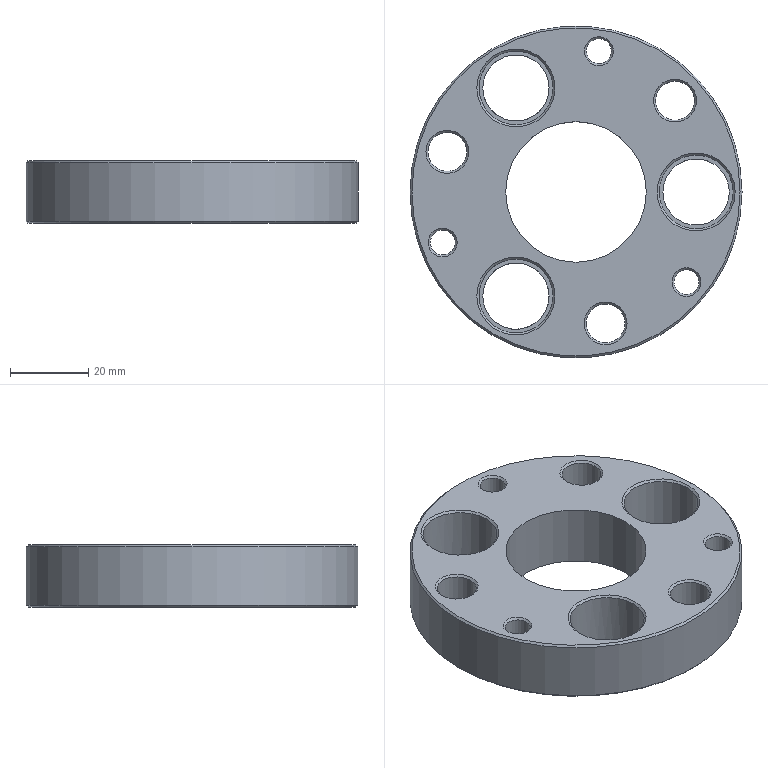Part | NX | features BREP 1 | 1 solid | 39 faces | box 85 x 85 x 16 mm | volume 54576 mm3 | cylinder 17 | cone 14 | plane 8 | commonest cylinder face diameters 6.4 x3 10 x3 10.5 x3 17 x3 19 x3 36 x1
STEP:
#1=CARTESIAN_POINT('',(-5.38,-26.639,16.));
#2=VERTEX_POINT('',#1);
#3=CARTESIAN_POINT('',(-15.38,-26.639,16.));
#4=DIRECTION('',(0.,0.,-1.));
#5=DIRECTION('',(1.,0.,0.));
#6=AXIS2_PLACEMENT_3D('',#3,#4,#5);
#7=CIRCLE('',#6,10.);
#8=EDGE_CURVE('',#2,#2,#7,.T.);
#9=ORIENTED_EDGE('',*,*,#8,.F.);
#10=EDGE_LOOP('',(#9));
#11=FACE_BOUND('',#10,.T.);
#12=CARTESIAN_POINT('',(-5.88,-26.639,15.5));
#13=VERTEX_POINT('',#12);
#14=CARTESIAN_POINT('',(-15.38,-26.639,15.5));
#15=DIRECTION('',(0.,0.,1.));
#16=DIRECTION('',(1.,0.,0.));
#17=AXIS2_PLACEMENT_3D('',#14,#15,#16);
#18=CIRCLE('',#17,9.5);
#19=EDGE_CURVE('',#13,#13,#18,.T.);
#20=ORIENTED_EDGE('',*,*,#19,.F.);
#21=EDGE_LOOP('',(#20));
#22=FACE_BOUND('',#21,.T.);
#23=CARTESIAN_POINT('',(-15.38,-26.639,16.));
#24=DIRECTION('',(0.,0.,1.));
#25=DIRECTION('',(1.,0.,0.));
#26=AXIS2_PLACEMENT_3D('',#23,#24,#25);
#27=CONICAL_SURFACE('',#26,10.,0.7854);
#28=ADVANCED_FACE('',(#11,#22),#27,.F.);
#29=CARTESIAN_POINT('',(-5.38,26.639,16.));
#30=VERTEX_POINT('',#29);
#31=CARTESIAN_POINT('',(-15.38,26.639,16.));
#32=DIRECTION('',(0.,0.,-1.));
#33=DIRECTION('',(1.,0.,0.));
#34=AXIS2_PLACEMENT_3D('',#31,#32,#33);
#35=CIRCLE('',#34,10.);
#36=EDGE_CURVE('',#30,#30,#35,.T.);
#37=ORIENTED_EDGE('',*,*,#36,.F.);
#38=EDGE_LOOP('',(#37));
#39=FACE_BOUND('',#38,.T.);
#40=CARTESIAN_POINT('',(-5.88,26.639,15.5));
#41=VERTEX_POINT('',#40);
#42=CARTESIAN_POINT('',(-15.38,26.639,15.5));
#43=DIRECTION('',(0.,0.,1.));
#44=DIRECTION('',(1.,0.,0.));
#45=AXIS2_PLACEMENT_3D('',#42,#43,#44);
#46=CIRCLE('',#45,9.5);
#47=EDGE_CURVE('',#41,#41,#46,.T.);
#48=ORIENTED_EDGE('',*,*,#47,.F.);
#49=EDGE_LOOP('',(#48));
#50=FACE_BOUND('',#49,.T.);
#51=CARTESIAN_POINT('',(-15.38,26.639,16.));
#52=DIRECTION('',(0.,0.,1.));
#53=DIRECTION('',(1.,0.,0.));
#54=AXIS2_PLACEMENT_3D('',#51,#52,#53);
#55=CONICAL_SURFACE('',#54,10.,0.7854);
#56=ADVANCED_FACE('',(#39,#50),#55,.F.);
#57=CARTESIAN_POINT('',(40.76,0.,16.));
#58=VERTEX_POINT('',#57);
#59=CARTESIAN_POINT('',(30.76,0.,16.));
#60=DIRECTION('',(0.,0.,-1.));
#61=DIRECTION('',(1.,0.,0.));
#62=AXIS2_PLACEMENT_3D('',#59,#60,#61);
#63=CIRCLE('',#62,10.);
#64=EDGE_CURVE('',#58,#58,#63,.T.);
#65=ORIENTED_EDGE('',*,*,#64,.F.);
#66=EDGE_LOOP('',(#65));
#67=FACE_BOUND('',#66,.T.);
#68=CARTESIAN_POINT('',(40.26,0.,15.5));
#69=VERTEX_POINT('',#68);
#70=CARTESIAN_POINT('',(30.76,0.,15.5));
#71=DIRECTION('',(0.,0.,1.));
#72=DIRECTION('',(1.,0.,0.));
#73=AXIS2_PLACEMENT_3D('',#70,#71,#72);
#74=CIRCLE('',#73,9.5);
#75=EDGE_CURVE('',#69,#69,#74,.T.);
#76=ORIENTED_EDGE('',*,*,#75,.F.);
#77=EDGE_LOOP('',(#76));
#78=FACE_BOUND('',#77,.T.);
#79=CARTESIAN_POINT('',(30.76,0.,16.));
#80=DIRECTION('',(0.,0.,1.));
#81=DIRECTION('',(1.,0.,0.));
#82=AXIS2_PLACEMENT_3D('',#79,#80,#81);
#83=CONICAL_SURFACE('',#82,10.,0.7854);
#84=ADVANCED_FACE('',(#67,#78),#83,.F.);
#85=CARTESIAN_POINT('',(0.5951,36.029,0.));
#86=VERTEX_POINT('',#85);
#87=CARTESIAN_POINT('',(5.845,36.029,0.));
#88=DIRECTION('',(0.,0.,-1.));
#89=DIRECTION('',(-1.,0.,0.));
#90=AXIS2_PLACEMENT_3D('',#87,#88,#89);
#91=CIRCLE('',#90,5.25);
#92=EDGE_CURVE('',#86,#86,#91,.T.);
#93=ORIENTED_EDGE('',*,*,#92,.T.);
#94=EDGE_LOOP('',(#93));
#95=FACE_BOUND('',#94,.T.);
#96=CARTESIAN_POINT('',(0.5951,36.029,7.5));
#97=VERTEX_POINT('',#96);
#98=CARTESIAN_POINT('',(5.845,36.029,7.5));
#99=DIRECTION('',(0.,0.,-1.));
#100=DIRECTION('',(-1.,0.,0.));
#101=AXIS2_PLACEMENT_3D('',#98,#99,#100);
#102=CIRCLE('',#101,5.25);
#103=EDGE_CURVE('',#97,#97,#102,.T.);
#104=ORIENTED_EDGE('',*,*,#103,.F.);
#105=EDGE_LOOP('',(#104));
#106=FACE_BOUND('',#105,.T.);
#107=CARTESIAN_POINT('',(5.845,36.029,0.));
#108=DIRECTION('',(0.,0.,-1.));
#109=DIRECTION('',(-1.,0.,0.));
#110=AXIS2_PLACEMENT_3D('',#107,#108,#109);
#111=CYLINDRICAL_SURFACE('',#110,5.25);
#112=ADVANCED_FACE('',(#95,#106),#111,.F.);
#113=CARTESIAN_POINT('',(-39.375,-12.952,0.));
#114=VERTEX_POINT('',#113);
#115=CARTESIAN_POINT('',(-34.125,-12.952,0.));
#116=DIRECTION('',(0.,0.,-1.));
#117=DIRECTION('',(-1.,0.,0.));
#118=AXIS2_PLACEMENT_3D('',#115,#116,#117);
#119=CIRCLE('',#118,5.25);
#120=EDGE_CURVE('',#114,#114,#119,.T.);
#121=ORIENTED_EDGE('',*,*,#120,.T.);
#122=EDGE_LOOP('',(#121));
#123=FACE_BOUND('',#122,.T.);
#124=CARTESIAN_POINT('',(-39.375,-12.952,7.5));
#125=VERTEX_POINT('',#124);
#126=CARTESIAN_POINT('',(-34.125,-12.952,7.5));
#127=DIRECTION('',(0.,0.,-1.));
#128=DIRECTION('',(-1.,0.,0.));
#129=AXIS2_PLACEMENT_3D('',#126,#127,#128);
#130=CIRCLE('',#129,5.25);
#131=EDGE_CURVE('',#125,#125,#130,.T.);
#132=ORIENTED_EDGE('',*,*,#131,.F.);
#133=EDGE_LOOP('',(#132));
#134=FACE_BOUND('',#133,.T.);
#135=CARTESIAN_POINT('',(-34.125,-12.952,0.));
#136=DIRECTION('',(0.,0.,-1.));
#137=DIRECTION('',(-1.,0.,0.));
#138=AXIS2_PLACEMENT_3D('',#135,#136,#137);
#139=CYLINDRICAL_SURFACE('',#138,5.25);
#140=ADVANCED_FACE('',(#123,#134),#139,.F.);
#141=CARTESIAN_POINT('',(23.029,-23.076,0.));
#142=VERTEX_POINT('',#141);
#143=CARTESIAN_POINT('',(28.279,-23.076,0.));
#144=DIRECTION('',(0.,0.,-1.));
#145=DIRECTION('',(-1.,0.,0.));
#146=AXIS2_PLACEMENT_3D('',#143,#144,#145);
#147=CIRCLE('',#146,5.25);
#148=EDGE_CURVE('',#142,#142,#147,.T.);
#149=ORIENTED_EDGE('',*,*,#148,.T.);
#150=EDGE_LOOP('',(#149));
#151=FACE_BOUND('',#150,.T.);
#152=CARTESIAN_POINT('',(23.029,-23.076,7.5));
#153=VERTEX_POINT('',#152);
#154=CARTESIAN_POINT('',(28.279,-23.076,7.5));
#155=DIRECTION('',(0.,0.,-1.));
#156=DIRECTION('',(-1.,0.,0.));
#157=AXIS2_PLACEMENT_3D('',#154,#155,#156);
#158=CIRCLE('',#157,5.25);
#159=EDGE_CURVE('',#153,#153,#158,.T.);
#160=ORIENTED_EDGE('',*,*,#159,.F.);
#161=EDGE_LOOP('',(#160));
#162=FACE_BOUND('',#161,.T.);
#163=CARTESIAN_POINT('',(28.279,-23.076,0.));
#164=DIRECTION('',(0.,0.,-1.));
#165=DIRECTION('',(-1.,0.,0.));
#166=AXIS2_PLACEMENT_3D('',#163,#164,#165);
#167=CYLINDRICAL_SURFACE('',#166,5.25);
#168=ADVANCED_FACE('',(#151,#162),#167,.F.);
#169=CARTESIAN_POINT('',(42.5,0.,0.5));
#170=VERTEX_POINT('',#169);
#171=CARTESIAN_POINT('',(0.,0.,0.5));
#172=DIRECTION('',(0.,0.,1.));
#173=DIRECTION('',(1.,0.,0.));
#174=AXIS2_PLACEMENT_3D('',#171,#172,#173);
#175=CIRCLE('',#174,42.5);
#176=EDGE_CURVE('',#170,#170,#175,.T.);
#177=ORIENTED_EDGE('',*,*,#176,.F.);
#178=EDGE_LOOP('',(#177));
#179=FACE_BOUND('',#178,.T.);
#180=CARTESIAN_POINT('',(42.,0.,0.));
#181=VERTEX_POINT('',#180);
#182=CARTESIAN_POINT('',(0.,0.,0.));
#183=DIRECTION('',(0.,0.,-1.));
#184=DIRECTION('',(1.,0.,0.));
#185=AXIS2_PLACEMENT_3D('',#182,#183,#184);
#186=CIRCLE('',#185,42.);
#187=EDGE_CURVE('',#181,#181,#186,.T.);
#188=ORIENTED_EDGE('',*,*,#187,.F.);
#189=EDGE_LOOP('',(#188));
#190=FACE_BOUND('',#189,.T.);
#191=CARTESIAN_POINT('',(0.,0.,0.5));
#192=DIRECTION('',(0.,0.,1.));
#193=DIRECTION('',(1.,0.,0.));
#194=AXIS2_PLACEMENT_3D('',#191,#192,#193);
#195=CONICAL_SURFACE('',#194,42.5,0.7854);
#196=ADVANCED_FACE('',(#179,#190),#195,.T.);
#197=CARTESIAN_POINT('',(42.5,0.,15.5));
#198=VERTEX_POINT('',#197);
#199=CARTESIAN_POINT('',(0.,0.,15.5));
#200=DIRECTION('',(0.,0.,-1.));
#201=DIRECTION('',(1.,0.,0.));
#202=AXIS2_PLACEMENT_3D('',#199,#200,#201);
#203=CIRCLE('',#202,42.5);
#204=EDGE_CURVE('',#198,#198,#203,.T.);
#205=ORIENTED_EDGE('',*,*,#204,.F.);
#206=EDGE_LOOP('',(#205));
#207=FACE_BOUND('',#206,.T.);
#208=CARTESIAN_POINT('',(42.,0.,16.));
#209=VERTEX_POINT('',#208);
#210=CARTESIAN_POINT('',(0.,0.,16.));
#211=DIRECTION('',(0.,0.,1.));
#212=DIRECTION('',(1.,0.,0.));
#213=AXIS2_PLACEMENT_3D('',#210,#211,#212);
#214=CIRCLE('',#213,42.);
#215=EDGE_CURVE('',#209,#209,#214,.T.);
#216=ORIENTED_EDGE('',*,*,#215,.F.);
#217=EDGE_LOOP('',(#216));
#218=FACE_BOUND('',#217,.T.);
#219=CARTESIAN_POINT('',(0.,0.,16.));
#220=DIRECTION('',(0.,0.,-1.));
#221=DIRECTION('',(-1.,0.,0.));
#222=AXIS2_PLACEMENT_3D('',#219,#220,#221);
#223=CONICAL_SURFACE('',#222,42.,0.7854);
#224=ADVANCED_FACE('',(#207,#218),#223,.T.);
#225=CARTESIAN_POINT('',(-27.427,10.265,0.));
#226=VERTEX_POINT('',#225);
#227=CARTESIAN_POINT('',(-32.927,10.265,0.));
#228=DIRECTION('',(0.,0.,1.));
#229=DIRECTION('',(1.,0.,0.));
#230=AXIS2_PLACEMENT_3D('',#227,#228,#229);
#231=CIRCLE('',#230,5.5);
#232=EDGE_CURVE('',#226,#226,#231,.T.);
#233=ORIENTED_EDGE('',*,*,#232,.F.);
#234=EDGE_LOOP('',(#233));
#235=FACE_BOUND('',#234,.T.);
#236=CARTESIAN_POINT('',(-27.927,10.265,0.5));
#237=VERTEX_POINT('',#236);
#238=CARTESIAN_POINT('',(-32.927,10.265,0.5));
#239=DIRECTION('',(0.,0.,-1.));
#240=DIRECTION('',(1.,0.,0.));
#241=AXIS2_PLACEMENT_3D('',#238,#239,#240);
#242=CIRCLE('',#241,5.);
#243=EDGE_CURVE('',#237,#237,#242,.T.);
#244=ORIENTED_EDGE('',*,*,#243,.F.);
#245=EDGE_LOOP('',(#244));
#246=FACE_BOUND('',#245,.T.);
#247=CARTESIAN_POINT('',(-32.927,10.265,0.5));
#248=DIRECTION('',(0.,0.,-1.));
#249=DIRECTION('',(-1.,0.,0.));
#250=AXIS2_PLACEMENT_3D('',#247,#248,#249);
#251=CONICAL_SURFACE('',#250,5.,0.7854);
#252=ADVANCED_FACE('',(#235,#246),#251,.F.);
#253=CARTESIAN_POINT('',(-27.427,10.265,16.));
#254=VERTEX_POINT('',#253);
#255=CARTESIAN_POINT('',(-32.927,10.265,16.));
#256=DIRECTION('',(0.,0.,-1.));
#257=DIRECTION('',(1.,0.,0.));
#258=AXIS2_PLACEMENT_3D('',#255,#256,#257);
#259=CIRCLE('',#258,5.5);
#260=EDGE_CURVE('',#254,#254,#259,.T.);
#261=ORIENTED_EDGE('',*,*,#260,.F.);
#262=EDGE_LOOP('',(#261));
#263=FACE_BOUND('',#262,.T.);
#264=CARTESIAN_POINT('',(-27.927,10.265,15.5));
#265=VERTEX_POINT('',#264);
#266=CARTESIAN_POINT('',(-32.927,10.265,15.5));
#267=DIRECTION('',(0.,0.,1.));
#268=DIRECTION('',(1.,0.,0.));
#269=AXIS2_PLACEMENT_3D('',#266,#267,#268);
#270=CIRCLE('',#269,5.);
#271=EDGE_CURVE('',#265,#265,#270,.T.);
#272=ORIENTED_EDGE('',*,*,#271,.F.);
#273=EDGE_LOOP('',(#272));
#274=FACE_BOUND('',#273,.T.);
#275=CARTESIAN_POINT('',(-32.927,10.265,16.));
#276=DIRECTION('',(0.,0.,1.));
#277=DIRECTION('',(1.,0.,0.));
#278=AXIS2_PLACEMENT_3D('',#275,#276,#277);
#279=CONICAL_SURFACE('',#278,5.5,0.7854);
#280=ADVANCED_FACE('',(#263,#274),#279,.F.);
#281=CARTESIAN_POINT('',(-30.425,-12.952,16.));
#282=VERTEX_POINT('',#281);
#283=CARTESIAN_POINT('',(-34.125,-12.952,16.));
#284=DIRECTION('',(0.,0.,-1.));
#285=DIRECTION('',(1.,0.,0.));
#286=AXIS2_PLACEMENT_3D('',#283,#284,#285);
#287=CIRCLE('',#286,3.7);
#288=EDGE_CURVE('',#282,#282,#287,.T.);
#289=ORIENTED_EDGE('',*,*,#288,.F.);
#290=EDGE_LOOP('',(#289));
#291=FACE_BOUND('',#290,.T.);
#292=CARTESIAN_POINT('',(-30.925,-12.952,15.5));
#293=VERTEX_POINT('',#292);
#294=CARTESIAN_POINT('',(-34.125,-12.952,15.5));
#295=DIRECTION('',(0.,0.,1.));
#296=DIRECTION('',(1.,0.,0.));
#297=AXIS2_PLACEMENT_3D('',#294,#295,#296);
#298=CIRCLE('',#297,3.2);
#299=EDGE_CURVE('',#293,#293,#298,.T.);
#300=ORIENTED_EDGE('',*,*,#299,.F.);
#301=EDGE_LOOP('',(#300));
#302=FACE_BOUND('',#301,.T.);
#303=CARTESIAN_POINT('',(-34.125,-12.952,16.));
#304=DIRECTION('',(0.,0.,1.));
#305=DIRECTION('',(1.,0.,0.));
#306=AXIS2_PLACEMENT_3D('',#303,#304,#305);
#307=CONICAL_SURFACE('',#306,3.7,0.7854);
#308=ADVANCED_FACE('',(#291,#302),#307,.F.);
#309=CARTESIAN_POINT('',(13.074,-33.648,0.));
#310=VERTEX_POINT('',#309);
#311=CARTESIAN_POINT('',(7.574,-33.648,0.));
#312=DIRECTION('',(0.,0.,1.));
#313=DIRECTION('',(1.,0.,0.));
#314=AXIS2_PLACEMENT_3D('',#311,#312,#313);
#315=CIRCLE('',#314,5.5);
#316=EDGE_CURVE('',#310,#310,#315,.T.);
#317=ORIENTED_EDGE('',*,*,#316,.F.);
#318=EDGE_LOOP('',(#317));
#319=FACE_BOUND('',#318,.T.);
#320=CARTESIAN_POINT('',(12.574,-33.648,0.5));
#321=VERTEX_POINT('',#320);
#322=CARTESIAN_POINT('',(7.574,-33.648,0.5));
#323=DIRECTION('',(0.,0.,-1.));
#324=DIRECTION('',(1.,0.,0.));
#325=AXIS2_PLACEMENT_3D('',#322,#323,#324);
#326=CIRCLE('',#325,5.);
#327=EDGE_CURVE('',#321,#321,#326,.T.);
#328=ORIENTED_EDGE('',*,*,#327,.F.);
#329=EDGE_LOOP('',(#328));
#330=FACE_BOUND('',#329,.T.);
#331=CARTESIAN_POINT('',(7.574,-33.648,0.5));
#332=DIRECTION('',(0.,0.,-1.));
#333=DIRECTION('',(-1.,0.,0.));
#334=AXIS2_PLACEMENT_3D('',#331,#332,#333);
#335=CONICAL_SURFACE('',#334,5.,0.7854);
#336=ADVANCED_FACE('',(#319,#330),#335,.F.);
#337=CARTESIAN_POINT('',(13.074,-33.648,16.));
#338=VERTEX_POINT('',#337);
#339=CARTESIAN_POINT('',(7.574,-33.648,16.));
#340=DIRECTION('',(0.,0.,-1.));
#341=DIRECTION('',(1.,0.,0.));
#342=AXIS2_PLACEMENT_3D('',#339,#340,#341);
#343=CIRCLE('',#342,5.5);
#344=EDGE_CURVE('',#338,#338,#343,.T.);
#345=ORIENTED_EDGE('',*,*,#344,.F.);
#346=EDGE_LOOP('',(#345));
#347=FACE_BOUND('',#346,.T.);
#348=CARTESIAN_POINT('',(12.574,-33.648,15.5));
#349=VERTEX_POINT('',#348);
#350=CARTESIAN_POINT('',(7.574,-33.648,15.5));
#351=DIRECTION('',(0.,0.,1.));
#352=DIRECTION('',(1.,0.,0.));
#353=AXIS2_PLACEMENT_3D('',#350,#351,#352);
#354=CIRCLE('',#353,5.);
#355=EDGE_CURVE('',#349,#349,#354,.T.);
#356=ORIENTED_EDGE('',*,*,#355,.F.);
#357=EDGE_LOOP('',(#356));
#358=FACE_BOUND('',#357,.T.);
#359=CARTESIAN_POINT('',(7.574,-33.648,16.));
#360=DIRECTION('',(0.,0.,1.));
#361=DIRECTION('',(1.,0.,0.));
#362=AXIS2_PLACEMENT_3D('',#359,#360,#361);
#363=CONICAL_SURFACE('',#362,5.5,0.7854);
#364=ADVANCED_FACE('',(#347,#358),#363,.F.);
#365=CARTESIAN_POINT('',(31.979,-23.076,16.));
#366=VERTEX_POINT('',#365);
#367=CARTESIAN_POINT('',(28.279,-23.076,16.));
#368=DIRECTION('',(0.,0.,-1.));
#369=DIRECTION('',(1.,0.,0.));
#370=AXIS2_PLACEMENT_3D('',#367,#368,#369);
#371=CIRCLE('',#370,3.7);
#372=EDGE_CURVE('',#366,#366,#371,.T.);
#373=ORIENTED_EDGE('',*,*,#372,.F.);
#374=EDGE_LOOP('',(#373));
#375=FACE_BOUND('',#374,.T.);
#376=CARTESIAN_POINT('',(31.479,-23.076,15.5));
#377=VERTEX_POINT('',#376);
#378=CARTESIAN_POINT('',(28.279,-23.076,15.5));
#379=DIRECTION('',(0.,0.,1.));
#380=DIRECTION('',(1.,0.,0.));
#381=AXIS2_PLACEMENT_3D('',#378,#379,#380);
#382=CIRCLE('',#381,3.2);
#383=EDGE_CURVE('',#377,#377,#382,.T.);
#384=ORIENTED_EDGE('',*,*,#383,.F.);
#385=EDGE_LOOP('',(#384));
#386=FACE_BOUND('',#385,.T.);
#387=CARTESIAN_POINT('',(28.279,-23.076,16.));
#388=DIRECTION('',(0.,0.,1.));
#389=DIRECTION('',(1.,0.,0.));
#390=AXIS2_PLACEMENT_3D('',#387,#388,#389);
#391=CONICAL_SURFACE('',#390,3.7,0.7854);
#392=ADVANCED_FACE('',(#375,#386),#391,.F.);
#393=ORIENTED_EDGE('',*,*,#47,.T.);
#394=EDGE_LOOP('',(#393));
#395=FACE_BOUND('',#394,.T.);
#396=CARTESIAN_POINT('',(-10.63,18.412,2.));
#397=VERTEX_POINT('',#396);
#398=CARTESIAN_POINT('',(-15.38,26.639,2.));
#399=DIRECTION('',(0.,0.,-1.));
#400=DIRECTION('',(0.5,-0.866,0.));
#401=AXIS2_PLACEMENT_3D('',#398,#399,#400);
#402=CIRCLE('',#401,9.5);
#403=EDGE_CURVE('',#397,#397,#402,.T.);
#404=ORIENTED_EDGE('',*,*,#403,.T.);
#405=EDGE_LOOP('',(#404));
#406=FACE_BOUND('',#405,.T.);
#407=CARTESIAN_POINT('',(-15.38,26.639,2.));
#408=DIRECTION('',(0.,0.,1.));
#409=DIRECTION('',(1.,0.,0.));
#410=AXIS2_PLACEMENT_3D('',#407,#408,#409);
#411=CYLINDRICAL_SURFACE('',#410,9.5);
#412=ADVANCED_FACE('',(#395,#406),#411,.F.);
#413=ORIENTED_EDGE('',*,*,#19,.T.);
#414=EDGE_LOOP('',(#413));
#415=FACE_BOUND('',#414,.T.);
#416=CARTESIAN_POINT('',(-10.63,-18.412,2.));
#417=VERTEX_POINT('',#416);
#418=CARTESIAN_POINT('',(-15.38,-26.639,2.));
#419=DIRECTION('',(0.,0.,-1.));
#420=DIRECTION('',(0.5,0.866,0.));
#421=AXIS2_PLACEMENT_3D('',#418,#419,#420);
#422=CIRCLE('',#421,9.5);
#423=EDGE_CURVE('',#417,#417,#422,.T.);
#424=ORIENTED_EDGE('',*,*,#423,.T.);
#425=EDGE_LOOP('',(#424));
#426=FACE_BOUND('',#425,.T.);
#427=CARTESIAN_POINT('',(-15.38,-26.639,2.));
#428=DIRECTION('',(0.,0.,1.));
#429=DIRECTION('',(1.,0.,0.));
#430=AXIS2_PLACEMENT_3D('',#427,#428,#429);
#431=CYLINDRICAL_SURFACE('',#430,9.5);
#432=ADVANCED_FACE('',(#415,#426),#431,.F.);
#433=CARTESIAN_POINT('',(-37.325,-12.952,7.5));
#434=VERTEX_POINT('',#433);
#435=CARTESIAN_POINT('',(-34.125,-12.952,7.5));
#436=DIRECTION('',(0.,0.,-1.));
#437=DIRECTION('',(-1.,0.,0.));
#438=AXIS2_PLACEMENT_3D('',#435,#436,#437);
#439=CIRCLE('',#438,3.2);
#440=EDGE_CURVE('',#434,#434,#439,.T.);
#441=ORIENTED_EDGE('',*,*,#440,.T.);
#442=EDGE_LOOP('',(#441));
#443=FACE_BOUND('',#442,.T.);
#444=ORIENTED_EDGE('',*,*,#299,.T.);
#445=EDGE_LOOP('',(#444));
#446=FACE_BOUND('',#445,.T.);
#447=CARTESIAN_POINT('',(-34.125,-12.952,16.));
#448=DIRECTION('',(0.,0.,-1.));
#449=DIRECTION('',(-1.,0.,0.));
#450=AXIS2_PLACEMENT_3D('',#447,#448,#449);
#451=CYLINDRICAL_SURFACE('',#450,3.2);
#452=ADVANCED_FACE('',(#443,#446),#451,.F.);
#453=ORIENTED_EDGE('',*,*,#243,.T.);
#454=EDGE_LOOP('',(#453));
#455=FACE_BOUND('',#454,.T.);
#456=ORIENTED_EDGE('',*,*,#271,.T.);
#457=EDGE_LOOP('',(#456));
#458=FACE_BOUND('',#457,.T.);
#459=CARTESIAN_POINT('',(-32.927,10.265,16.));
#460=DIRECTION('',(0.,0.,-1.));
#461=DIRECTION('',(-1.,0.,0.));
#462=AXIS2_PLACEMENT_3D('',#459,#460,#461);
#463=CYLINDRICAL_SURFACE('',#462,5.);
#464=ADVANCED_FACE('',(#455,#458),#463,.F.);
#465=CARTESIAN_POINT('',(-11.13,19.278,0.));
#466=VERTEX_POINT('',#465);
#467=CARTESIAN_POINT('',(-15.38,26.639,0.));
#468=DIRECTION('',(0.,0.,-1.));
#469=DIRECTION('',(0.5,-0.866,0.));
#470=AXIS2_PLACEMENT_3D('',#467,#468,#469);
#471=CIRCLE('',#470,8.5);
#472=EDGE_CURVE('',#466,#466,#471,.T.);
#473=ORIENTED_EDGE('',*,*,#472,.T.);
#474=EDGE_LOOP('',(#473));
#475=FACE_BOUND('',#474,.T.);
#476=CARTESIAN_POINT('',(-23.88,26.639,2.));
#477=VERTEX_POINT('',#476);
#478=CARTESIAN_POINT('',(-15.38,26.639,2.));
#479=DIRECTION('',(0.,0.,1.));
#480=DIRECTION('',(-1.,0.,0.));
#481=AXIS2_PLACEMENT_3D('',#478,#479,#480);
#482=CIRCLE('',#481,8.5);
#483=EDGE_CURVE('',#477,#477,#482,.T.);
#484=ORIENTED_EDGE('',*,*,#483,.T.);
#485=EDGE_LOOP('',(#484));
#486=FACE_BOUND('',#485,.T.);
#487=CARTESIAN_POINT('',(-15.38,26.639,16.));
#488=DIRECTION('',(0.,0.,-1.));
#489=DIRECTION('',(-1.,0.,0.));
#490=AXIS2_PLACEMENT_3D('',#487,#488,#489);
#491=CYLINDRICAL_SURFACE('',#490,8.5);
#492=ADVANCED_FACE('',(#475,#486),#491,.F.);
#493=CARTESIAN_POINT('',(25.079,-23.076,7.5));
#494=VERTEX_POINT('',#493);
#495=CARTESIAN_POINT('',(28.279,-23.076,7.5));
#496=DIRECTION('',(0.,0.,-1.));
#497=DIRECTION('',(-1.,0.,0.));
#498=AXIS2_PLACEMENT_3D('',#495,#496,#497);
#499=CIRCLE('',#498,3.2);
#500=EDGE_CURVE('',#494,#494,#499,.T.);
#501=ORIENTED_EDGE('',*,*,#500,.T.);
#502=EDGE_LOOP('',(#501));
#503=FACE_BOUND('',#502,.T.);
#504=ORIENTED_EDGE('',*,*,#383,.T.);
#505=EDGE_LOOP('',(#504));
#506=FACE_BOUND('',#505,.T.);
#507=CARTESIAN_POINT('',(28.279,-23.076,16.));
#508=DIRECTION('',(0.,0.,-1.));
#509=DIRECTION('',(-1.,0.,0.));
#510=AXIS2_PLACEMENT_3D('',#507,#508,#509);
#511=CYLINDRICAL_SURFACE('',#510,3.2);
#512=ADVANCED_FACE('',(#503,#506),#511,.F.);
#513=ORIENTED_EDGE('',*,*,#327,.T.);
#514=EDGE_LOOP('',(#513));
#515=FACE_BOUND('',#514,.T.);
#516=ORIENTED_EDGE('',*,*,#355,.T.);
#517=EDGE_LOOP('',(#516));
#518=FACE_BOUND('',#517,.T.);
#519=CARTESIAN_POINT('',(7.574,-33.648,16.));
#520=DIRECTION('',(0.,0.,-1.));
#521=DIRECTION('',(-1.,0.,0.));
#522=AXIS2_PLACEMENT_3D('',#519,#520,#521);
#523=CYLINDRICAL_SURFACE('',#522,5.);
#524=ADVANCED_FACE('',(#515,#518),#523,.F.);
#525=CARTESIAN_POINT('',(-11.13,-19.278,0.));
#526=VERTEX_POINT('',#525);
#527=CARTESIAN_POINT('',(-15.38,-26.639,0.));
#528=DIRECTION('',(0.,0.,-1.));
#529=DIRECTION('',(0.5,0.866,0.));
#530=AXIS2_PLACEMENT_3D('',#527,#528,#529);
#531=CIRCLE('',#530,8.5);
#532=EDGE_CURVE('',#526,#526,#531,.T.);
#533=ORIENTED_EDGE('',*,*,#532,.T.);
#534=EDGE_LOOP('',(#533));
#535=FACE_BOUND('',#534,.T.);
#536=CARTESIAN_POINT('',(-23.88,-26.639,2.));
#537=VERTEX_POINT('',#536);
#538=CARTESIAN_POINT('',(-15.38,-26.639,2.));
#539=DIRECTION('',(0.,0.,1.));
#540=DIRECTION('',(-1.,0.,0.));
#541=AXIS2_PLACEMENT_3D('',#538,#539,#540);
#542=CIRCLE('',#541,8.5);
#543=EDGE_CURVE('',#537,#537,#542,.T.);
#544=ORIENTED_EDGE('',*,*,#543,.T.);
#545=EDGE_LOOP('',(#544));
#546=FACE_BOUND('',#545,.T.);
#547=CARTESIAN_POINT('',(-15.38,-26.639,16.));
#548=DIRECTION('',(0.,0.,-1.));
#549=DIRECTION('',(-1.,0.,0.));
#550=AXIS2_PLACEMENT_3D('',#547,#548,#549);
#551=CYLINDRICAL_SURFACE('',#550,8.5);
#552=ADVANCED_FACE('',(#535,#546),#551,.F.);
#553=CARTESIAN_POINT('',(30.853,23.383,0.));
#554=VERTEX_POINT('',#553);
#555=CARTESIAN_POINT('',(25.353,23.383,0.));
#556=DIRECTION('',(0.,0.,1.));
#557=DIRECTION('',(1.,0.,0.));
#558=AXIS2_PLACEMENT_3D('',#555,#556,#557);
#559=CIRCLE('',#558,5.5);
#560=EDGE_CURVE('',#554,#554,#559,.T.);
#561=ORIENTED_EDGE('',*,*,#560,.F.);
#562=EDGE_LOOP('',(#561));
#563=FACE_BOUND('',#562,.T.);
#564=CARTESIAN_POINT('',(30.353,23.383,0.5));
#565=VERTEX_POINT('',#564);
#566=CARTESIAN_POINT('',(25.353,23.383,0.5));
#567=DIRECTION('',(0.,0.,-1.));
#568=DIRECTION('',(1.,0.,0.));
#569=AXIS2_PLACEMENT_3D('',#566,#567,#568);
#570=CIRCLE('',#569,5.);
#571=EDGE_CURVE('',#565,#565,#570,.T.);
#572=ORIENTED_EDGE('',*,*,#571,.F.);
#573=EDGE_LOOP('',(#572));
#574=FACE_BOUND('',#573,.T.);
#575=CARTESIAN_POINT('',(25.353,23.383,0.5));
#576=DIRECTION('',(0.,0.,-1.));
#577=DIRECTION('',(-1.,0.,0.));
#578=AXIS2_PLACEMENT_3D('',#575,#576,#577);
#579=CONICAL_SURFACE('',#578,5.,0.7854);
#580=ADVANCED_FACE('',(#563,#574),#579,.F.);
#581=CARTESIAN_POINT('',(30.853,23.383,16.));
#582=VERTEX_POINT('',#581);
#583=CARTESIAN_POINT('',(25.353,23.383,16.));
#584=DIRECTION('',(0.,0.,-1.));
#585=DIRECTION('',(1.,0.,0.));
#586=AXIS2_PLACEMENT_3D('',#583,#584,#585);
#587=CIRCLE('',#586,5.5);
#588=EDGE_CURVE('',#582,#582,#587,.T.);
#589=ORIENTED_EDGE('',*,*,#588,.F.);
#590=EDGE_LOOP('',(#589));
#591=FACE_BOUND('',#590,.T.);
#592=CARTESIAN_POINT('',(30.353,23.383,15.5));
#593=VERTEX_POINT('',#592);
#594=CARTESIAN_POINT('',(25.353,23.383,15.5));
#595=DIRECTION('',(0.,0.,1.));
#596=DIRECTION('',(1.,0.,0.));
#597=AXIS2_PLACEMENT_3D('',#594,#595,#596);
#598=CIRCLE('',#597,5.);
#599=EDGE_CURVE('',#593,#593,#598,.T.);
#600=ORIENTED_EDGE('',*,*,#599,.F.);
#601=EDGE_LOOP('',(#600));
#602=FACE_BOUND('',#601,.T.);
#603=CARTESIAN_POINT('',(25.353,23.383,16.));
#604=DIRECTION('',(0.,0.,1.));
#605=DIRECTION('',(1.,0.,0.));
#606=AXIS2_PLACEMENT_3D('',#603,#604,#605);
#607=CONICAL_SURFACE('',#606,5.5,0.7854);
#608=ADVANCED_FACE('',(#591,#602),#607,.F.);
#609=CARTESIAN_POINT('',(9.545,36.029,16.));
#610=VERTEX_POINT('',#609);
#611=CARTESIAN_POINT('',(5.845,36.029,16.));
#612=DIRECTION('',(0.,0.,-1.));
#613=DIRECTION('',(1.,0.,0.));
#614=AXIS2_PLACEMENT_3D('',#611,#612,#613);
#615=CIRCLE('',#614,3.7);
#616=EDGE_CURVE('',#610,#610,#615,.T.);
#617=ORIENTED_EDGE('',*,*,#616,.F.);
#618=EDGE_LOOP('',(#617));
#619=FACE_BOUND('',#618,.T.);
#620=CARTESIAN_POINT('',(9.045,36.029,15.5));
#621=VERTEX_POINT('',#620);
#622=CARTESIAN_POINT('',(5.845,36.029,15.5));
#623=DIRECTION('',(0.,0.,1.));
#624=DIRECTION('',(1.,0.,0.));
#625=AXIS2_PLACEMENT_3D('',#622,#623,#624);
#626=CIRCLE('',#625,3.2);
#627=EDGE_CURVE('',#621,#621,#626,.T.);
#628=ORIENTED_EDGE('',*,*,#627,.F.);
#629=EDGE_LOOP('',(#628));
#630=FACE_BOUND('',#629,.T.);
#631=CARTESIAN_POINT('',(5.845,36.029,16.));
#632=DIRECTION('',(0.,0.,1.));
#633=DIRECTION('',(1.,0.,0.));
#634=AXIS2_PLACEMENT_3D('',#631,#632,#633);
#635=CONICAL_SURFACE('',#634,3.7,0.7854);
#636=ADVANCED_FACE('',(#619,#630),#635,.F.);
#637=ORIENTED_EDGE('',*,*,#75,.T.);
#638=EDGE_LOOP('',(#637));
#639=FACE_BOUND('',#638,.T.);
#640=CARTESIAN_POINT('',(21.26,0.,2.));
#641=VERTEX_POINT('',#640);
#642=CARTESIAN_POINT('',(30.76,0.,2.));
#643=DIRECTION('',(0.,0.,-1.));
#644=DIRECTION('',(-1.,0.,0.));
#645=AXIS2_PLACEMENT_3D('',#642,#643,#644);
#646=CIRCLE('',#645,9.5);
#647=EDGE_CURVE('',#641,#641,#646,.T.);
#648=ORIENTED_EDGE('',*,*,#647,.T.);
#649=EDGE_LOOP('',(#648));
#650=FACE_BOUND('',#649,.T.);
#651=CARTESIAN_POINT('',(30.76,0.,2.));
#652=DIRECTION('',(0.,0.,1.));
#653=DIRECTION('',(1.,0.,0.));
#654=AXIS2_PLACEMENT_3D('',#651,#652,#653);
#655=CYLINDRICAL_SURFACE('',#654,9.5);
#656=ADVANCED_FACE('',(#639,#650),#655,.F.);
#657=CARTESIAN_POINT('',(2.645,36.029,7.5));
#658=VERTEX_POINT('',#657);
#659=CARTESIAN_POINT('',(5.845,36.029,7.5));
#660=DIRECTION('',(0.,0.,-1.));
#661=DIRECTION('',(-1.,0.,0.));
#662=AXIS2_PLACEMENT_3D('',#659,#660,#661);
#663=CIRCLE('',#662,3.2);
#664=EDGE_CURVE('',#658,#658,#663,.T.);
#665=ORIENTED_EDGE('',*,*,#664,.T.);
#666=EDGE_LOOP('',(#665));
#667=FACE_BOUND('',#666,.T.);
#668=ORIENTED_EDGE('',*,*,#627,.T.);
#669=EDGE_LOOP('',(#668));
#670=FACE_BOUND('',#669,.T.);
#671=CARTESIAN_POINT('',(5.845,36.029,16.));
#672=DIRECTION('',(0.,0.,-1.));
#673=DIRECTION('',(-1.,0.,0.));
#674=AXIS2_PLACEMENT_3D('',#671,#672,#673);
#675=CYLINDRICAL_SURFACE('',#674,3.2);
#676=ADVANCED_FACE('',(#667,#670),#675,.F.);
#677=ORIENTED_EDGE('',*,*,#571,.T.);
#678=EDGE_LOOP('',(#677));
#679=FACE_BOUND('',#678,.T.);
#680=ORIENTED_EDGE('',*,*,#599,.T.);
#681=EDGE_LOOP('',(#680));
#682=FACE_BOUND('',#681,.T.);
#683=CARTESIAN_POINT('',(25.353,23.383,16.));
#684=DIRECTION('',(0.,0.,-1.));
#685=DIRECTION('',(-1.,0.,0.));
#686=AXIS2_PLACEMENT_3D('',#683,#684,#685);
#687=CYLINDRICAL_SURFACE('',#686,5.);
#688=ADVANCED_FACE('',(#679,#682),#687,.F.);
#689=CARTESIAN_POINT('',(22.26,0.,0.));
#690=VERTEX_POINT('',#689);
#691=CARTESIAN_POINT('',(30.76,0.,0.));
#692=DIRECTION('',(0.,0.,-1.));
#693=DIRECTION('',(-1.,0.,0.));
#694=AXIS2_PLACEMENT_3D('',#691,#692,#693);
#695=CIRCLE('',#694,8.5);
#696=EDGE_CURVE('',#690,#690,#695,.T.);
#697=ORIENTED_EDGE('',*,*,#696,.T.);
#698=EDGE_LOOP('',(#697));
#699=FACE_BOUND('',#698,.T.);
#700=CARTESIAN_POINT('',(22.26,0.,2.));
#701=VERTEX_POINT('',#700);
#702=CARTESIAN_POINT('',(30.76,0.,2.));
#703=DIRECTION('',(0.,0.,1.));
#704=DIRECTION('',(-1.,0.,0.));
#705=AXIS2_PLACEMENT_3D('',#702,#703,#704);
#706=CIRCLE('',#705,8.5);
#707=EDGE_CURVE('',#701,#701,#706,.T.);
#708=ORIENTED_EDGE('',*,*,#707,.T.);
#709=EDGE_LOOP('',(#708));
#710=FACE_BOUND('',#709,.T.);
#711=CARTESIAN_POINT('',(30.76,0.,16.));
#712=DIRECTION('',(0.,0.,-1.));
#713=DIRECTION('',(-1.,0.,0.));
#714=AXIS2_PLACEMENT_3D('',#711,#712,#713);
#715=CYLINDRICAL_SURFACE('',#714,8.5);
#716=ADVANCED_FACE('',(#699,#710),#715,.F.);
#717=CARTESIAN_POINT('',(18.,0.,0.));
#718=VERTEX_POINT('',#717);
#719=CARTESIAN_POINT('',(0.,0.,0.));
#720=DIRECTION('',(0.,0.,1.));
#721=DIRECTION('',(1.,0.,0.));
#722=AXIS2_PLACEMENT_3D('',#719,#720,#721);
#723=CIRCLE('',#722,18.);
#724=EDGE_CURVE('',#718,#718,#723,.T.);
#725=ORIENTED_EDGE('',*,*,#724,.F.);
#726=EDGE_LOOP('',(#725));
#727=FACE_BOUND('',#726,.T.);
#728=CARTESIAN_POINT('',(18.,0.,16.));
#729=VERTEX_POINT('',#728);
#730=CARTESIAN_POINT('',(0.,0.,16.));
#731=DIRECTION('',(0.,0.,1.));
#732=DIRECTION('',(1.,0.,0.));
#733=AXIS2_PLACEMENT_3D('',#730,#731,#732);
#734=CIRCLE('',#733,18.);
#735=EDGE_CURVE('',#729,#729,#734,.T.);
#736=ORIENTED_EDGE('',*,*,#735,.T.);
#737=EDGE_LOOP('',(#736));
#738=FACE_BOUND('',#737,.T.);
#739=CARTESIAN_POINT('',(0.,0.,16.));
#740=DIRECTION('',(0.,0.,-1.));
#741=DIRECTION('',(-1.,0.,0.));
#742=AXIS2_PLACEMENT_3D('',#739,#740,#741);
#743=CYLINDRICAL_SURFACE('',#742,18.);
#744=ADVANCED_FACE('',(#727,#738),#743,.F.);
#745=ORIENTED_EDGE('',*,*,#176,.T.);
#746=EDGE_LOOP('',(#745));
#747=FACE_BOUND('',#746,.T.);
#748=ORIENTED_EDGE('',*,*,#204,.T.);
#749=EDGE_LOOP('',(#748));
#750=FACE_BOUND('',#749,.T.);
#751=CARTESIAN_POINT('',(0.,0.,16.));
#752=DIRECTION('',(0.,0.,-1.));
#753=DIRECTION('',(-1.,0.,0.));
#754=AXIS2_PLACEMENT_3D('',#751,#752,#753);
#755=CYLINDRICAL_SURFACE('',#754,42.5);
#756=ADVANCED_FACE('',(#747,#750),#755,.T.);
#757=ORIENTED_EDGE('',*,*,#64,.T.);
#758=EDGE_LOOP('',(#757));
#759=FACE_BOUND('',#758,.T.);
#760=ORIENTED_EDGE('',*,*,#36,.T.);
#761=EDGE_LOOP('',(#760));
#762=FACE_BOUND('',#761,.T.);
#763=ORIENTED_EDGE('',*,*,#8,.T.);
#764=EDGE_LOOP('',(#763));
#765=FACE_BOUND('',#764,.T.);
#766=ORIENTED_EDGE('',*,*,#215,.T.);
#767=EDGE_LOOP('',(#766));
#768=FACE_BOUND('',#767,.T.);
#769=ORIENTED_EDGE('',*,*,#288,.T.);
#770=EDGE_LOOP('',(#769));
#771=FACE_BOUND('',#770,.T.);
#772=ORIENTED_EDGE('',*,*,#260,.T.);
#773=EDGE_LOOP('',(#772));
#774=FACE_BOUND('',#773,.T.);
#775=ORIENTED_EDGE('',*,*,#372,.T.);
#776=EDGE_LOOP('',(#775));
#777=FACE_BOUND('',#776,.T.);
#778=ORIENTED_EDGE('',*,*,#344,.T.);
#779=EDGE_LOOP('',(#778));
#780=FACE_BOUND('',#779,.T.);
#781=ORIENTED_EDGE('',*,*,#616,.T.);
#782=EDGE_LOOP('',(#781));
#783=FACE_BOUND('',#782,.T.);
#784=ORIENTED_EDGE('',*,*,#588,.T.);
#785=EDGE_LOOP('',(#784));
#786=FACE_BOUND('',#785,.T.);
#787=ORIENTED_EDGE('',*,*,#735,.F.);
#788=EDGE_LOOP('',(#787));
#789=FACE_BOUND('',#788,.T.);
#790=CARTESIAN_POINT('',(0.,0.,16.));
#791=DIRECTION('',(0.,0.,1.));
#792=DIRECTION('',(1.,0.,0.));
#793=AXIS2_PLACEMENT_3D('',#790,#791,#792);
#794=PLANE('',#793);
#795=ADVANCED_FACE('',(#759,#762,#765,#768,#771,#774,#777,#780,#783,#786,#789),#794,.T.);
#796=ORIENTED_EDGE('',*,*,#92,.F.);
#797=EDGE_LOOP('',(#796));
#798=FACE_BOUND('',#797,.T.);
#799=ORIENTED_EDGE('',*,*,#120,.F.);
#800=EDGE_LOOP('',(#799));
#801=FACE_BOUND('',#800,.T.);
#802=ORIENTED_EDGE('',*,*,#148,.F.);
#803=EDGE_LOOP('',(#802));
#804=FACE_BOUND('',#803,.T.);
#805=ORIENTED_EDGE('',*,*,#187,.T.);
#806=EDGE_LOOP('',(#805));
#807=FACE_BOUND('',#806,.T.);
#808=ORIENTED_EDGE('',*,*,#232,.T.);
#809=EDGE_LOOP('',(#808));
#810=FACE_BOUND('',#809,.T.);
#811=ORIENTED_EDGE('',*,*,#316,.T.);
#812=EDGE_LOOP('',(#811));
#813=FACE_BOUND('',#812,.T.);
#814=ORIENTED_EDGE('',*,*,#472,.F.);
#815=EDGE_LOOP('',(#814));
#816=FACE_BOUND('',#815,.T.);
#817=ORIENTED_EDGE('',*,*,#532,.F.);
#818=EDGE_LOOP('',(#817));
#819=FACE_BOUND('',#818,.T.);
#820=ORIENTED_EDGE('',*,*,#560,.T.);
#821=EDGE_LOOP('',(#820));
#822=FACE_BOUND('',#821,.T.);
#823=ORIENTED_EDGE('',*,*,#696,.F.);
#824=EDGE_LOOP('',(#823));
#825=FACE_BOUND('',#824,.T.);
#826=ORIENTED_EDGE('',*,*,#724,.T.);
#827=EDGE_LOOP('',(#826));
#828=FACE_BOUND('',#827,.T.);
#829=CARTESIAN_POINT('',(0.,0.,0.));
#830=DIRECTION('',(0.,0.,1.));
#831=DIRECTION('',(1.,0.,0.));
#832=AXIS2_PLACEMENT_3D('',#829,#830,#831);
#833=PLANE('',#832);
#834=ADVANCED_FACE('',(#798,#801,#804,#807,#810,#813,#816,#819,#822,#825,#828),#833,.F.);
#835=ORIENTED_EDGE('',*,*,#647,.F.);
#836=EDGE_LOOP('',(#835));
#837=FACE_BOUND('',#836,.T.);
#838=ORIENTED_EDGE('',*,*,#707,.F.);
#839=EDGE_LOOP('',(#838));
#840=FACE_BOUND('',#839,.T.);
#841=CARTESIAN_POINT('',(30.76,0.,2.));
#842=DIRECTION('',(0.,0.,-1.));
#843=DIRECTION('',(-1.,0.,0.));
#844=AXIS2_PLACEMENT_3D('',#841,#842,#843);
#845=PLANE('',#844);
#846=ADVANCED_FACE('',(#837,#840),#845,.F.);
#847=ORIENTED_EDGE('',*,*,#423,.F.);
#848=EDGE_LOOP('',(#847));
#849=FACE_BOUND('',#848,.T.);
#850=ORIENTED_EDGE('',*,*,#543,.F.);
#851=EDGE_LOOP('',(#850));
#852=FACE_BOUND('',#851,.T.);
#853=CARTESIAN_POINT('',(-15.38,-26.639,2.));
#854=DIRECTION('',(0.,0.,-1.));
#855=DIRECTION('',(0.5,0.866,0.));
#856=AXIS2_PLACEMENT_3D('',#853,#854,#855);
#857=PLANE('',#856);
#858=ADVANCED_FACE('',(#849,#852),#857,.F.);
#859=ORIENTED_EDGE('',*,*,#403,.F.);
#860=EDGE_LOOP('',(#859));
#861=FACE_BOUND('',#860,.T.);
#862=ORIENTED_EDGE('',*,*,#483,.F.);
#863=EDGE_LOOP('',(#862));
#864=FACE_BOUND('',#863,.T.);
#865=CARTESIAN_POINT('',(-15.38,26.639,2.));
#866=DIRECTION('',(0.,0.,-1.));
#867=DIRECTION('',(0.5,-0.866,0.));
#868=AXIS2_PLACEMENT_3D('',#865,#866,#867);
#869=PLANE('',#868);
#870=ADVANCED_FACE('',(#861,#864),#869,.F.);
#871=ORIENTED_EDGE('',*,*,#500,.F.);
#872=EDGE_LOOP('',(#871));
#873=FACE_BOUND('',#872,.T.);
#874=ORIENTED_EDGE('',*,*,#159,.T.);
#875=EDGE_LOOP('',(#874));
#876=FACE_BOUND('',#875,.T.);
#877=CARTESIAN_POINT('',(31.479,-23.076,7.5));
#878=DIRECTION('',(0.,0.,1.));
#879=DIRECTION('',(1.,0.,0.));
#880=AXIS2_PLACEMENT_3D('',#877,#878,#879);
#881=PLANE('',#880);
#882=ADVANCED_FACE('',(#873,#876),#881,.F.);
#883=ORIENTED_EDGE('',*,*,#440,.F.);
#884=EDGE_LOOP('',(#883));
#885=FACE_BOUND('',#884,.T.);
#886=ORIENTED_EDGE('',*,*,#131,.T.);
#887=EDGE_LOOP('',(#886));
#888=FACE_BOUND('',#887,.T.);
#889=CARTESIAN_POINT('',(-30.925,-12.952,7.5));
#890=DIRECTION('',(0.,0.,1.));
#891=DIRECTION('',(1.,0.,0.));
#892=AXIS2_PLACEMENT_3D('',#889,#890,#891);
#893=PLANE('',#892);
#894=ADVANCED_FACE('',(#885,#888),#893,.F.);
#895=ORIENTED_EDGE('',*,*,#664,.F.);
#896=EDGE_LOOP('',(#895));
#897=FACE_BOUND('',#896,.T.);
#898=ORIENTED_EDGE('',*,*,#103,.T.);
#899=EDGE_LOOP('',(#898));
#900=FACE_BOUND('',#899,.T.);
#901=CARTESIAN_POINT('',(9.045,36.029,7.5));
#902=DIRECTION('',(0.,0.,1.));
#903=DIRECTION('',(1.,0.,0.));
#904=AXIS2_PLACEMENT_3D('',#901,#902,#903);
#905=PLANE('',#904);
#906=ADVANCED_FACE('',(#897,#900),#905,.F.);
#907=CLOSED_SHELL('',(#28,#56,#84,#112,#140,#168,#196,#224,#252,#280,#308,#336,#364,#392,#412,#432,#452,#464,#492,#512,#524,#552,#580,#608,#636,#656,#676,#688,#716,#744,#756,#795,#834,#846,#858,#870,#882,#894,#906));
#908=MANIFOLD_SOLID_BREP('',#907);
#909=(LENGTH_UNIT()NAMED_UNIT(*)SI_UNIT(.MILLI.,.METRE.));
#910=UNCERTAINTY_MEASURE_WITH_UNIT(LENGTH_MEASURE(0.00001),#909,'','');
#911=(NAMED_UNIT(*)PLANE_ANGLE_UNIT()SI_UNIT($,.RADIAN.));
#912=(NAMED_UNIT(*)SI_UNIT($,.STERADIAN.)SOLID_ANGLE_UNIT());
#913=(GEOMETRIC_REPRESENTATION_CONTEXT(3)GLOBAL_UNCERTAINTY_ASSIGNED_CONTEXT((#910))GLOBAL_UNIT_ASSIGNED_CONTEXT((#909,#911,#912))REPRESENTATION_CONTEXT('',''));
#914=ADVANCED_BREP_SHAPE_REPRESENTATION('',(#908),#913);